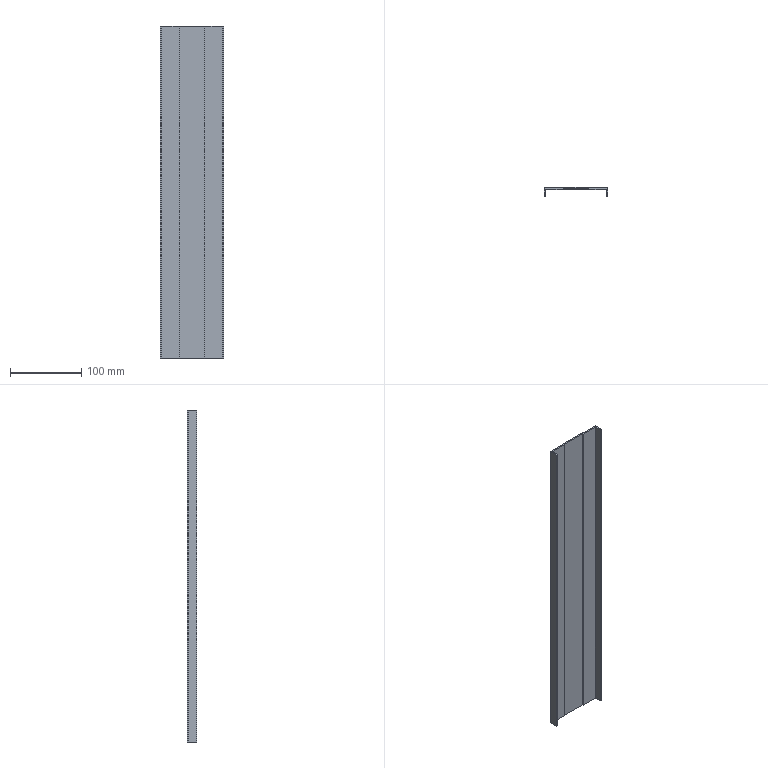Part | NX | 1 solid | 18 faces | box 89 x 13 x 466 mm | volume 103452 mm3 | plane 18
STEP:
#1=CARTESIAN_POINT('',(42.5,10.,-233.));
#2=VERTEX_POINT('',#1);
#3=CARTESIAN_POINT('',(42.5,0.,-233.));
#4=VERTEX_POINT('',#3);
#5=CARTESIAN_POINT('',(42.5,12.,-233.));
#6=DIRECTION('',(0.,-1.,0.));
#7=VECTOR('',#6,1000.);
#8=LINE('',#5,#7);
#9=EDGE_CURVE('',#2,#4,#8,.T.);
#10=ORIENTED_EDGE('',*,*,#9,.T.);
#11=CARTESIAN_POINT('',(42.5,0.,233.));
#12=VERTEX_POINT('',#11);
#13=CARTESIAN_POINT('',(42.5,0.,233.));
#14=DIRECTION('',(0.,0.,-1.));
#15=VECTOR('',#14,1000.);
#16=LINE('',#13,#15);
#17=EDGE_CURVE('',#12,#4,#16,.T.);
#18=ORIENTED_EDGE('',*,*,#17,.F.);
#19=CARTESIAN_POINT('',(42.5,10.,233.));
#20=VERTEX_POINT('',#19);
#21=CARTESIAN_POINT('',(42.5,12.,233.));
#22=DIRECTION('',(0.,-1.,0.));
#23=VECTOR('',#22,1000.);
#24=LINE('',#21,#23);
#25=EDGE_CURVE('',#20,#12,#24,.T.);
#26=ORIENTED_EDGE('',*,*,#25,.F.);
#27=CARTESIAN_POINT('',(42.5,10.,233.));
#28=DIRECTION('',(0.,0.,-1.));
#29=VECTOR('',#28,1000.);
#30=LINE('',#27,#29);
#31=EDGE_CURVE('',#20,#2,#30,.T.);
#32=ORIENTED_EDGE('',*,*,#31,.T.);
#33=EDGE_LOOP('',(#10,#18,#26,#32));
#34=FACE_BOUND('',#33,.T.);
#35=CARTESIAN_POINT('',(42.5,12.,233.));
#36=DIRECTION('',(1.,0.,0.));
#37=DIRECTION('',(0.,1.,0.));
#38=AXIS2_PLACEMENT_3D('',#35,#36,#37);
#39=PLANE('',#38);
#40=ADVANCED_FACE('',(#34),#39,.F.);
#41=CARTESIAN_POINT('',(44.5,0.,-233.));
#42=VERTEX_POINT('',#41);
#43=CARTESIAN_POINT('',(44.5,0.,-233.));
#44=DIRECTION('',(-1.,0.,0.));
#45=VECTOR('',#44,1000.);
#46=LINE('',#43,#45);
#47=EDGE_CURVE('',#42,#4,#46,.T.);
#48=ORIENTED_EDGE('',*,*,#47,.F.);
#49=CARTESIAN_POINT('',(44.5,0.,233.));
#50=VERTEX_POINT('',#49);
#51=CARTESIAN_POINT('',(44.5,0.,233.));
#52=DIRECTION('',(0.,0.,-1.));
#53=VECTOR('',#52,1000.);
#54=LINE('',#51,#53);
#55=EDGE_CURVE('',#50,#42,#54,.T.);
#56=ORIENTED_EDGE('',*,*,#55,.F.);
#57=CARTESIAN_POINT('',(44.5,0.,233.));
#58=DIRECTION('',(-1.,0.,0.));
#59=VECTOR('',#58,1000.);
#60=LINE('',#57,#59);
#61=EDGE_CURVE('',#50,#12,#60,.T.);
#62=ORIENTED_EDGE('',*,*,#61,.T.);
#63=ORIENTED_EDGE('',*,*,#17,.T.);
#64=EDGE_LOOP('',(#48,#56,#62,#63));
#65=FACE_BOUND('',#64,.T.);
#66=CARTESIAN_POINT('',(44.5,0.,233.));
#67=DIRECTION('',(0.,-1.,0.));
#68=DIRECTION('',(1.,0.,0.));
#69=AXIS2_PLACEMENT_3D('',#66,#67,#68);
#70=PLANE('',#69);
#71=ADVANCED_FACE('',(#65),#70,.T.);
#72=CARTESIAN_POINT('',(44.5,12.,-233.));
#73=VERTEX_POINT('',#72);
#74=CARTESIAN_POINT('',(44.5,12.,-233.));
#75=DIRECTION('',(0.,-1.,0.));
#76=VECTOR('',#75,1000.);
#77=LINE('',#74,#76);
#78=EDGE_CURVE('',#73,#42,#77,.T.);
#79=ORIENTED_EDGE('',*,*,#78,.F.);
#80=CARTESIAN_POINT('',(44.5,12.,233.));
#81=VERTEX_POINT('',#80);
#82=CARTESIAN_POINT('',(44.5,12.,233.));
#83=DIRECTION('',(0.,0.,-1.));
#84=VECTOR('',#83,1000.);
#85=LINE('',#82,#84);
#86=EDGE_CURVE('',#81,#73,#85,.T.);
#87=ORIENTED_EDGE('',*,*,#86,.F.);
#88=CARTESIAN_POINT('',(44.5,12.,233.));
#89=DIRECTION('',(0.,-1.,0.));
#90=VECTOR('',#89,1000.);
#91=LINE('',#88,#90);
#92=EDGE_CURVE('',#81,#50,#91,.T.);
#93=ORIENTED_EDGE('',*,*,#92,.T.);
#94=ORIENTED_EDGE('',*,*,#55,.T.);
#95=EDGE_LOOP('',(#79,#87,#93,#94));
#96=FACE_BOUND('',#95,.T.);
#97=CARTESIAN_POINT('',(44.5,12.,233.));
#98=DIRECTION('',(1.,0.,0.));
#99=DIRECTION('',(0.,1.,0.));
#100=AXIS2_PLACEMENT_3D('',#97,#98,#99);
#101=PLANE('',#100);
#102=ADVANCED_FACE('',(#96),#101,.T.);
#103=CARTESIAN_POINT('',(20.,12.,-233.));
#104=VERTEX_POINT('',#103);
#105=CARTESIAN_POINT('',(20.,12.,-233.));
#106=DIRECTION('',(1.,0.,0.));
#107=VECTOR('',#106,1000.);
#108=LINE('',#105,#107);
#109=EDGE_CURVE('',#104,#73,#108,.T.);
#110=ORIENTED_EDGE('',*,*,#109,.F.);
#111=CARTESIAN_POINT('',(20.,12.,233.));
#112=VERTEX_POINT('',#111);
#113=CARTESIAN_POINT('',(20.,12.,233.));
#114=DIRECTION('',(0.,0.,-1.));
#115=VECTOR('',#114,1000.);
#116=LINE('',#113,#115);
#117=EDGE_CURVE('',#112,#104,#116,.T.);
#118=ORIENTED_EDGE('',*,*,#117,.F.);
#119=CARTESIAN_POINT('',(20.,12.,233.));
#120=DIRECTION('',(1.,0.,0.));
#121=VECTOR('',#120,1000.);
#122=LINE('',#119,#121);
#123=EDGE_CURVE('',#112,#81,#122,.T.);
#124=ORIENTED_EDGE('',*,*,#123,.T.);
#125=ORIENTED_EDGE('',*,*,#86,.T.);
#126=EDGE_LOOP('',(#110,#118,#124,#125));
#127=FACE_BOUND('',#126,.T.);
#128=CARTESIAN_POINT('',(20.,12.,233.));
#129=DIRECTION('',(0.,1.,0.));
#130=DIRECTION('',(-1.,0.,0.));
#131=AXIS2_PLACEMENT_3D('',#128,#129,#130);
#132=PLANE('',#131);
#133=ADVANCED_FACE('',(#127),#132,.T.);
#134=CARTESIAN_POINT('',(20.,13.,-233.));
#135=VERTEX_POINT('',#134);
#136=CARTESIAN_POINT('',(20.,13.,-233.));
#137=DIRECTION('',(0.,-1.,0.));
#138=VECTOR('',#137,1000.);
#139=LINE('',#136,#138);
#140=EDGE_CURVE('',#135,#104,#139,.T.);
#141=ORIENTED_EDGE('',*,*,#140,.F.);
#142=CARTESIAN_POINT('',(20.,13.,233.));
#143=VERTEX_POINT('',#142);
#144=CARTESIAN_POINT('',(20.,13.,233.));
#145=DIRECTION('',(0.,0.,-1.));
#146=VECTOR('',#145,1000.);
#147=LINE('',#144,#146);
#148=EDGE_CURVE('',#143,#135,#147,.T.);
#149=ORIENTED_EDGE('',*,*,#148,.F.);
#150=CARTESIAN_POINT('',(20.,13.,233.));
#151=DIRECTION('',(0.,-1.,0.));
#152=VECTOR('',#151,1000.);
#153=LINE('',#150,#152);
#154=EDGE_CURVE('',#143,#112,#153,.T.);
#155=ORIENTED_EDGE('',*,*,#154,.T.);
#156=ORIENTED_EDGE('',*,*,#117,.T.);
#157=EDGE_LOOP('',(#141,#149,#155,#156));
#158=FACE_BOUND('',#157,.T.);
#159=CARTESIAN_POINT('',(20.,13.,233.));
#160=DIRECTION('',(1.,0.,0.));
#161=DIRECTION('',(0.,0.,-1.));
#162=AXIS2_PLACEMENT_3D('',#159,#160,#161);
#163=PLANE('',#162);
#164=ADVANCED_FACE('',(#158),#163,.T.);
#165=CARTESIAN_POINT('',(-20.,13.,-233.));
#166=VERTEX_POINT('',#165);
#167=CARTESIAN_POINT('',(-20.,13.,-233.));
#168=DIRECTION('',(1.,0.,0.));
#169=VECTOR('',#168,1000.);
#170=LINE('',#167,#169);
#171=EDGE_CURVE('',#166,#135,#170,.T.);
#172=ORIENTED_EDGE('',*,*,#171,.F.);
#173=CARTESIAN_POINT('',(-20.,13.,233.));
#174=VERTEX_POINT('',#173);
#175=CARTESIAN_POINT('',(-20.,13.,233.));
#176=DIRECTION('',(0.,0.,-1.));
#177=VECTOR('',#176,1000.);
#178=LINE('',#175,#177);
#179=EDGE_CURVE('',#174,#166,#178,.T.);
#180=ORIENTED_EDGE('',*,*,#179,.F.);
#181=CARTESIAN_POINT('',(-20.,13.,233.));
#182=DIRECTION('',(1.,0.,0.));
#183=VECTOR('',#182,1000.);
#184=LINE('',#181,#183);
#185=EDGE_CURVE('',#174,#143,#184,.T.);
#186=ORIENTED_EDGE('',*,*,#185,.T.);
#187=ORIENTED_EDGE('',*,*,#148,.T.);
#188=EDGE_LOOP('',(#172,#180,#186,#187));
#189=FACE_BOUND('',#188,.T.);
#190=CARTESIAN_POINT('',(-20.,13.,233.));
#191=DIRECTION('',(0.,1.,0.));
#192=DIRECTION('',(-1.,0.,0.));
#193=AXIS2_PLACEMENT_3D('',#190,#191,#192);
#194=PLANE('',#193);
#195=ADVANCED_FACE('',(#189),#194,.T.);
#196=CARTESIAN_POINT('',(-20.,12.,-233.));
#197=VERTEX_POINT('',#196);
#198=CARTESIAN_POINT('',(-20.,12.,-233.));
#199=DIRECTION('',(0.,1.,0.));
#200=VECTOR('',#199,1000.);
#201=LINE('',#198,#200);
#202=EDGE_CURVE('',#197,#166,#201,.T.);
#203=ORIENTED_EDGE('',*,*,#202,.F.);
#204=CARTESIAN_POINT('',(-20.,12.,233.));
#205=VERTEX_POINT('',#204);
#206=CARTESIAN_POINT('',(-20.,12.,233.));
#207=DIRECTION('',(0.,0.,-1.));
#208=VECTOR('',#207,1000.);
#209=LINE('',#206,#208);
#210=EDGE_CURVE('',#205,#197,#209,.T.);
#211=ORIENTED_EDGE('',*,*,#210,.F.);
#212=CARTESIAN_POINT('',(-20.,12.,233.));
#213=DIRECTION('',(0.,1.,0.));
#214=VECTOR('',#213,1000.);
#215=LINE('',#212,#214);
#216=EDGE_CURVE('',#205,#174,#215,.T.);
#217=ORIENTED_EDGE('',*,*,#216,.T.);
#218=ORIENTED_EDGE('',*,*,#179,.T.);
#219=EDGE_LOOP('',(#203,#211,#217,#218));
#220=FACE_BOUND('',#219,.T.);
#221=CARTESIAN_POINT('',(-20.,12.,233.));
#222=DIRECTION('',(-1.,0.,0.));
#223=DIRECTION('',(0.,0.,1.));
#224=AXIS2_PLACEMENT_3D('',#221,#222,#223);
#225=PLANE('',#224);
#226=ADVANCED_FACE('',(#220),#225,.T.);
#227=CARTESIAN_POINT('',(-44.5,12.,-233.));
#228=VERTEX_POINT('',#227);
#229=CARTESIAN_POINT('',(-44.5,12.,-233.));
#230=DIRECTION('',(1.,0.,0.));
#231=VECTOR('',#230,1000.);
#232=LINE('',#229,#231);
#233=EDGE_CURVE('',#228,#197,#232,.T.);
#234=ORIENTED_EDGE('',*,*,#233,.F.);
#235=CARTESIAN_POINT('',(-44.5,12.,233.));
#236=VERTEX_POINT('',#235);
#237=CARTESIAN_POINT('',(-44.5,12.,233.));
#238=DIRECTION('',(0.,0.,-1.));
#239=VECTOR('',#238,1000.);
#240=LINE('',#237,#239);
#241=EDGE_CURVE('',#236,#228,#240,.T.);
#242=ORIENTED_EDGE('',*,*,#241,.F.);
#243=CARTESIAN_POINT('',(-44.5,12.,233.));
#244=DIRECTION('',(1.,0.,0.));
#245=VECTOR('',#244,1000.);
#246=LINE('',#243,#245);
#247=EDGE_CURVE('',#236,#205,#246,.T.);
#248=ORIENTED_EDGE('',*,*,#247,.T.);
#249=ORIENTED_EDGE('',*,*,#210,.T.);
#250=EDGE_LOOP('',(#234,#242,#248,#249));
#251=FACE_BOUND('',#250,.T.);
#252=CARTESIAN_POINT('',(-44.5,12.,233.));
#253=DIRECTION('',(0.,1.,0.));
#254=DIRECTION('',(0.,0.,1.));
#255=AXIS2_PLACEMENT_3D('',#252,#253,#254);
#256=PLANE('',#255);
#257=ADVANCED_FACE('',(#251),#256,.T.);
#258=CARTESIAN_POINT('',(-44.5,0.,-233.));
#259=VERTEX_POINT('',#258);
#260=CARTESIAN_POINT('',(-44.5,0.,-233.));
#261=DIRECTION('',(0.,1.,0.));
#262=VECTOR('',#261,1000.);
#263=LINE('',#260,#262);
#264=EDGE_CURVE('',#259,#228,#263,.T.);
#265=ORIENTED_EDGE('',*,*,#264,.F.);
#266=CARTESIAN_POINT('',(-44.5,0.,233.));
#267=VERTEX_POINT('',#266);
#268=CARTESIAN_POINT('',(-44.5,0.,233.));
#269=DIRECTION('',(0.,0.,-1.));
#270=VECTOR('',#269,1000.);
#271=LINE('',#268,#270);
#272=EDGE_CURVE('',#267,#259,#271,.T.);
#273=ORIENTED_EDGE('',*,*,#272,.F.);
#274=CARTESIAN_POINT('',(-44.5,0.,233.));
#275=DIRECTION('',(0.,1.,0.));
#276=VECTOR('',#275,1000.);
#277=LINE('',#274,#276);
#278=EDGE_CURVE('',#267,#236,#277,.T.);
#279=ORIENTED_EDGE('',*,*,#278,.T.);
#280=ORIENTED_EDGE('',*,*,#241,.T.);
#281=EDGE_LOOP('',(#265,#273,#279,#280));
#282=FACE_BOUND('',#281,.T.);
#283=CARTESIAN_POINT('',(-44.5,0.,233.));
#284=DIRECTION('',(-1.,0.,0.));
#285=DIRECTION('',(0.,0.,1.));
#286=AXIS2_PLACEMENT_3D('',#283,#284,#285);
#287=PLANE('',#286);
#288=ADVANCED_FACE('',(#282),#287,.T.);
#289=CARTESIAN_POINT('',(-42.5,0.,-233.));
#290=VERTEX_POINT('',#289);
#291=CARTESIAN_POINT('',(-42.5,0.,-233.));
#292=DIRECTION('',(-1.,0.,0.));
#293=VECTOR('',#292,1000.);
#294=LINE('',#291,#293);
#295=EDGE_CURVE('',#290,#259,#294,.T.);
#296=ORIENTED_EDGE('',*,*,#295,.F.);
#297=CARTESIAN_POINT('',(-42.5,0.,233.));
#298=VERTEX_POINT('',#297);
#299=CARTESIAN_POINT('',(-42.5,0.,233.));
#300=DIRECTION('',(0.,0.,-1.));
#301=VECTOR('',#300,1000.);
#302=LINE('',#299,#301);
#303=EDGE_CURVE('',#298,#290,#302,.T.);
#304=ORIENTED_EDGE('',*,*,#303,.F.);
#305=CARTESIAN_POINT('',(-42.5,0.,233.));
#306=DIRECTION('',(-1.,0.,0.));
#307=VECTOR('',#306,1000.);
#308=LINE('',#305,#307);
#309=EDGE_CURVE('',#298,#267,#308,.T.);
#310=ORIENTED_EDGE('',*,*,#309,.T.);
#311=ORIENTED_EDGE('',*,*,#272,.T.);
#312=EDGE_LOOP('',(#296,#304,#310,#311));
#313=FACE_BOUND('',#312,.T.);
#314=CARTESIAN_POINT('',(-42.5,0.,233.));
#315=DIRECTION('',(0.,-1.,0.));
#316=DIRECTION('',(0.,0.,-1.));
#317=AXIS2_PLACEMENT_3D('',#314,#315,#316);
#318=PLANE('',#317);
#319=ADVANCED_FACE('',(#313),#318,.T.);
#320=CARTESIAN_POINT('',(-42.5,10.,-233.));
#321=VERTEX_POINT('',#320);
#322=CARTESIAN_POINT('',(-42.5,0.,-233.));
#323=DIRECTION('',(0.,1.,0.));
#324=VECTOR('',#323,1000.);
#325=LINE('',#322,#324);
#326=EDGE_CURVE('',#290,#321,#325,.T.);
#327=ORIENTED_EDGE('',*,*,#326,.T.);
#328=CARTESIAN_POINT('',(-42.5,10.,233.));
#329=VERTEX_POINT('',#328);
#330=CARTESIAN_POINT('',(-42.5,10.,233.));
#331=DIRECTION('',(0.,0.,-1.));
#332=VECTOR('',#331,1000.);
#333=LINE('',#330,#332);
#334=EDGE_CURVE('',#329,#321,#333,.T.);
#335=ORIENTED_EDGE('',*,*,#334,.F.);
#336=CARTESIAN_POINT('',(-42.5,0.,233.));
#337=DIRECTION('',(0.,1.,0.));
#338=VECTOR('',#337,1000.);
#339=LINE('',#336,#338);
#340=EDGE_CURVE('',#298,#329,#339,.T.);
#341=ORIENTED_EDGE('',*,*,#340,.F.);
#342=ORIENTED_EDGE('',*,*,#303,.T.);
#343=EDGE_LOOP('',(#327,#335,#341,#342));
#344=FACE_BOUND('',#343,.T.);
#345=CARTESIAN_POINT('',(-42.5,0.,233.));
#346=DIRECTION('',(-1.,0.,0.));
#347=DIRECTION('',(0.,0.,1.));
#348=AXIS2_PLACEMENT_3D('',#345,#346,#347);
#349=PLANE('',#348);
#350=ADVANCED_FACE('',(#344),#349,.F.);
#351=CARTESIAN_POINT('',(-18.,10.,-233.));
#352=VERTEX_POINT('',#351);
#353=CARTESIAN_POINT('',(-44.5,10.,-233.));
#354=DIRECTION('',(1.,0.,0.));
#355=VECTOR('',#354,1000.);
#356=LINE('',#353,#355);
#357=EDGE_CURVE('',#321,#352,#356,.T.);
#358=ORIENTED_EDGE('',*,*,#357,.T.);
#359=CARTESIAN_POINT('',(-18.,10.,233.));
#360=VERTEX_POINT('',#359);
#361=CARTESIAN_POINT('',(-18.,10.,233.));
#362=DIRECTION('',(0.,0.,-1.));
#363=VECTOR('',#362,1000.);
#364=LINE('',#361,#363);
#365=EDGE_CURVE('',#360,#352,#364,.T.);
#366=ORIENTED_EDGE('',*,*,#365,.F.);
#367=CARTESIAN_POINT('',(-44.5,10.,233.));
#368=DIRECTION('',(1.,0.,0.));
#369=VECTOR('',#368,1000.);
#370=LINE('',#367,#369);
#371=EDGE_CURVE('',#329,#360,#370,.T.);
#372=ORIENTED_EDGE('',*,*,#371,.F.);
#373=ORIENTED_EDGE('',*,*,#334,.T.);
#374=EDGE_LOOP('',(#358,#366,#372,#373));
#375=FACE_BOUND('',#374,.T.);
#376=CARTESIAN_POINT('',(-44.5,10.,233.));
#377=DIRECTION('',(0.,1.,0.));
#378=DIRECTION('',(0.,0.,1.));
#379=AXIS2_PLACEMENT_3D('',#376,#377,#378);
#380=PLANE('',#379);
#381=ADVANCED_FACE('',(#375),#380,.F.);
#382=CARTESIAN_POINT('',(-18.,11.,-233.));
#383=VERTEX_POINT('',#382);
#384=CARTESIAN_POINT('',(-18.,12.,-233.));
#385=DIRECTION('',(0.,1.,0.));
#386=VECTOR('',#385,1000.);
#387=LINE('',#384,#386);
#388=EDGE_CURVE('',#352,#383,#387,.T.);
#389=ORIENTED_EDGE('',*,*,#388,.T.);
#390=CARTESIAN_POINT('',(-18.,11.,233.));
#391=VERTEX_POINT('',#390);
#392=CARTESIAN_POINT('',(-18.,11.,233.));
#393=DIRECTION('',(0.,0.,-1.));
#394=VECTOR('',#393,1000.);
#395=LINE('',#392,#394);
#396=EDGE_CURVE('',#391,#383,#395,.T.);
#397=ORIENTED_EDGE('',*,*,#396,.F.);
#398=CARTESIAN_POINT('',(-18.,12.,233.));
#399=DIRECTION('',(0.,1.,0.));
#400=VECTOR('',#399,1000.);
#401=LINE('',#398,#400);
#402=EDGE_CURVE('',#360,#391,#401,.T.);
#403=ORIENTED_EDGE('',*,*,#402,.F.);
#404=ORIENTED_EDGE('',*,*,#365,.T.);
#405=EDGE_LOOP('',(#389,#397,#403,#404));
#406=FACE_BOUND('',#405,.T.);
#407=CARTESIAN_POINT('',(-18.,12.,233.));
#408=DIRECTION('',(-1.,0.,0.));
#409=DIRECTION('',(0.,0.,1.));
#410=AXIS2_PLACEMENT_3D('',#407,#408,#409);
#411=PLANE('',#410);
#412=ADVANCED_FACE('',(#406),#411,.F.);
#413=CARTESIAN_POINT('',(18.,11.,-233.));
#414=VERTEX_POINT('',#413);
#415=CARTESIAN_POINT('',(-20.,11.,-233.));
#416=DIRECTION('',(1.,0.,0.));
#417=VECTOR('',#416,1000.);
#418=LINE('',#415,#417);
#419=EDGE_CURVE('',#383,#414,#418,.T.);
#420=ORIENTED_EDGE('',*,*,#419,.T.);
#421=CARTESIAN_POINT('',(18.,11.,233.));
#422=VERTEX_POINT('',#421);
#423=CARTESIAN_POINT('',(18.,11.,233.));
#424=DIRECTION('',(0.,0.,-1.));
#425=VECTOR('',#424,1000.);
#426=LINE('',#423,#425);
#427=EDGE_CURVE('',#422,#414,#426,.T.);
#428=ORIENTED_EDGE('',*,*,#427,.F.);
#429=CARTESIAN_POINT('',(-20.,11.,233.));
#430=DIRECTION('',(1.,0.,0.));
#431=VECTOR('',#430,1000.);
#432=LINE('',#429,#431);
#433=EDGE_CURVE('',#391,#422,#432,.T.);
#434=ORIENTED_EDGE('',*,*,#433,.F.);
#435=ORIENTED_EDGE('',*,*,#396,.T.);
#436=EDGE_LOOP('',(#420,#428,#434,#435));
#437=FACE_BOUND('',#436,.T.);
#438=CARTESIAN_POINT('',(-20.,11.,233.));
#439=DIRECTION('',(0.,1.,0.));
#440=DIRECTION('',(-1.,0.,0.));
#441=AXIS2_PLACEMENT_3D('',#438,#439,#440);
#442=PLANE('',#441);
#443=ADVANCED_FACE('',(#437),#442,.F.);
#444=CARTESIAN_POINT('',(18.,10.,-233.));
#445=VERTEX_POINT('',#444);
#446=CARTESIAN_POINT('',(18.,13.,-233.));
#447=DIRECTION('',(0.,1.,0.));
#448=VECTOR('',#447,1000.);
#449=LINE('',#446,#448);
#450=EDGE_CURVE('',#414,#445,#449,.F.);
#451=ORIENTED_EDGE('',*,*,#450,.T.);
#452=CARTESIAN_POINT('',(18.,10.,233.));
#453=VERTEX_POINT('',#452);
#454=CARTESIAN_POINT('',(18.,10.,233.));
#455=DIRECTION('',(0.,0.,-1.));
#456=VECTOR('',#455,1000.);
#457=LINE('',#454,#456);
#458=EDGE_CURVE('',#453,#445,#457,.T.);
#459=ORIENTED_EDGE('',*,*,#458,.F.);
#460=CARTESIAN_POINT('',(18.,13.,233.));
#461=DIRECTION('',(0.,1.,0.));
#462=VECTOR('',#461,1000.);
#463=LINE('',#460,#462);
#464=EDGE_CURVE('',#422,#453,#463,.F.);
#465=ORIENTED_EDGE('',*,*,#464,.F.);
#466=ORIENTED_EDGE('',*,*,#427,.T.);
#467=EDGE_LOOP('',(#451,#459,#465,#466));
#468=FACE_BOUND('',#467,.T.);
#469=CARTESIAN_POINT('',(18.,13.,233.));
#470=DIRECTION('',(1.,0.,0.));
#471=DIRECTION('',(0.,0.,-1.));
#472=AXIS2_PLACEMENT_3D('',#469,#470,#471);
#473=PLANE('',#472);
#474=ADVANCED_FACE('',(#468),#473,.F.);
#475=CARTESIAN_POINT('',(20.,10.,-233.));
#476=DIRECTION('',(1.,0.,0.));
#477=VECTOR('',#476,1000.);
#478=LINE('',#475,#477);
#479=EDGE_CURVE('',#445,#2,#478,.T.);
#480=ORIENTED_EDGE('',*,*,#479,.T.);
#481=ORIENTED_EDGE('',*,*,#31,.F.);
#482=CARTESIAN_POINT('',(20.,10.,233.));
#483=DIRECTION('',(1.,0.,0.));
#484=VECTOR('',#483,1000.);
#485=LINE('',#482,#484);
#486=EDGE_CURVE('',#453,#20,#485,.T.);
#487=ORIENTED_EDGE('',*,*,#486,.F.);
#488=ORIENTED_EDGE('',*,*,#458,.T.);
#489=EDGE_LOOP('',(#480,#481,#487,#488));
#490=FACE_BOUND('',#489,.T.);
#491=CARTESIAN_POINT('',(20.,10.,233.));
#492=DIRECTION('',(0.,1.,0.));
#493=DIRECTION('',(-1.,0.,0.));
#494=AXIS2_PLACEMENT_3D('',#491,#492,#493);
#495=PLANE('',#494);
#496=ADVANCED_FACE('',(#490),#495,.F.);
#497=ORIENTED_EDGE('',*,*,#25,.T.);
#498=ORIENTED_EDGE('',*,*,#61,.F.);
#499=ORIENTED_EDGE('',*,*,#92,.F.);
#500=ORIENTED_EDGE('',*,*,#123,.F.);
#501=ORIENTED_EDGE('',*,*,#154,.F.);
#502=ORIENTED_EDGE('',*,*,#185,.F.);
#503=ORIENTED_EDGE('',*,*,#216,.F.);
#504=ORIENTED_EDGE('',*,*,#247,.F.);
#505=ORIENTED_EDGE('',*,*,#278,.F.);
#506=ORIENTED_EDGE('',*,*,#309,.F.);
#507=ORIENTED_EDGE('',*,*,#340,.T.);
#508=ORIENTED_EDGE('',*,*,#371,.T.);
#509=ORIENTED_EDGE('',*,*,#402,.T.);
#510=ORIENTED_EDGE('',*,*,#433,.T.);
#511=ORIENTED_EDGE('',*,*,#464,.T.);
#512=ORIENTED_EDGE('',*,*,#486,.T.);
#513=EDGE_LOOP('',(#497,#498,#499,#500,#501,#502,#503,#504,#505,#506,#507,#508,#509,#510,#511,#512));
#514=FACE_BOUND('',#513,.T.);
#515=CARTESIAN_POINT('',(0.,0.,233.));
#516=DIRECTION('',(0.,0.,-1.));
#517=DIRECTION('',(-1.,0.,0.));
#518=AXIS2_PLACEMENT_3D('',#515,#516,#517);
#519=PLANE('',#518);
#520=ADVANCED_FACE('',(#514),#519,.F.);
#521=ORIENTED_EDGE('',*,*,#9,.F.);
#522=ORIENTED_EDGE('',*,*,#479,.F.);
#523=ORIENTED_EDGE('',*,*,#450,.F.);
#524=ORIENTED_EDGE('',*,*,#419,.F.);
#525=ORIENTED_EDGE('',*,*,#388,.F.);
#526=ORIENTED_EDGE('',*,*,#357,.F.);
#527=ORIENTED_EDGE('',*,*,#326,.F.);
#528=ORIENTED_EDGE('',*,*,#295,.T.);
#529=ORIENTED_EDGE('',*,*,#264,.T.);
#530=ORIENTED_EDGE('',*,*,#233,.T.);
#531=ORIENTED_EDGE('',*,*,#202,.T.);
#532=ORIENTED_EDGE('',*,*,#171,.T.);
#533=ORIENTED_EDGE('',*,*,#140,.T.);
#534=ORIENTED_EDGE('',*,*,#109,.T.);
#535=ORIENTED_EDGE('',*,*,#78,.T.);
#536=ORIENTED_EDGE('',*,*,#47,.T.);
#537=EDGE_LOOP('',(#521,#522,#523,#524,#525,#526,#527,#528,#529,#530,#531,#532,#533,#534,#535,#536));
#538=FACE_BOUND('',#537,.T.);
#539=CARTESIAN_POINT('',(0.,0.,-233.));
#540=DIRECTION('',(0.,0.,-1.));
#541=DIRECTION('',(-1.,0.,0.));
#542=AXIS2_PLACEMENT_3D('',#539,#540,#541);
#543=PLANE('',#542);
#544=ADVANCED_FACE('',(#538),#543,.T.);
#545=CLOSED_SHELL('',(#40,#71,#102,#133,#164,#195,#226,#257,#288,#319,#350,#381,#412,#443,#474,#496,#520,#544));
#546=MANIFOLD_SOLID_BREP('',#545);
#547=(LENGTH_UNIT()NAMED_UNIT(*)SI_UNIT(.MILLI.,.METRE.));
#548=UNCERTAINTY_MEASURE_WITH_UNIT(LENGTH_MEASURE(0.00001),#547,'','');
#549=(NAMED_UNIT(*)PLANE_ANGLE_UNIT()SI_UNIT($,.RADIAN.));
#550=(NAMED_UNIT(*)SI_UNIT($,.STERADIAN.)SOLID_ANGLE_UNIT());
#551=(GEOMETRIC_REPRESENTATION_CONTEXT(3)GLOBAL_UNCERTAINTY_ASSIGNED_CONTEXT((#548))GLOBAL_UNIT_ASSIGNED_CONTEXT((#547,#549,#550))REPRESENTATION_CONTEXT('',''));
#552=ADVANCED_BREP_SHAPE_REPRESENTATION('',(#546),#551);